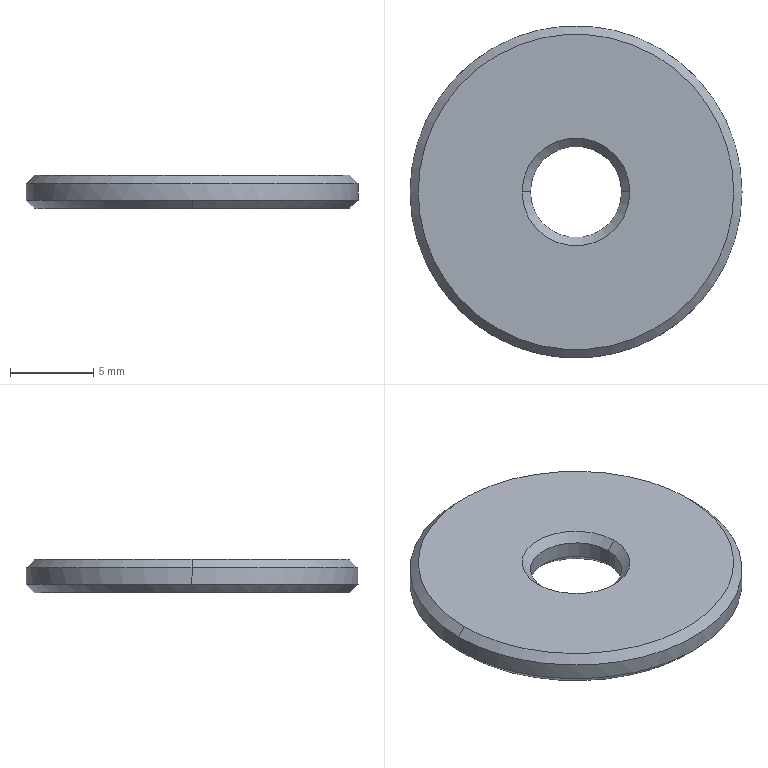Part | SolidWorks | features BaseBody 1 | 1 solid | 14 faces | box 20 x 20 x 2 mm | volume 560.774 mm3 | cone 8 | cylinder 4 | plane 2 | commonest cylinder face diameters 5.5 x2 20 x2
STEP:
#1=CARTESIAN_POINT('',(0.,9.5,-2.));
#2=VERTEX_POINT('',#1);
#3=CARTESIAN_POINT('',(0.,-9.5,-2.));
#4=VERTEX_POINT('',#3);
#5=CARTESIAN_POINT('',(0.,0.,-2.));
#6=DIRECTION('',(0.,0.,-1.));
#7=DIRECTION('',(0.,-1.,0.));
#8=AXIS2_PLACEMENT_3D('',#5,#6,#7);
#9=CIRCLE('',#8,9.5);
#10=EDGE_CURVE('',#2,#4,#9,.T.);
#11=ORIENTED_EDGE('',*,*,#10,.F.);
#12=CARTESIAN_POINT('',(0.,10.,-1.5));
#13=VERTEX_POINT('',#12);
#14=CARTESIAN_POINT('',(0.,10.,-1.5));
#15=DIRECTION('',(0.,0.7071,0.7071));
#16=VECTOR('',#15,1000.);
#17=LINE('',#14,#16);
#18=EDGE_CURVE('',#2,#13,#17,.T.);
#19=ORIENTED_EDGE('',*,*,#18,.T.);
#20=CARTESIAN_POINT('',(10.,0.,-1.5));
#21=VERTEX_POINT('',#20);
#22=CARTESIAN_POINT('',(0.,0.,-1.5));
#23=DIRECTION('',(0.,0.,-1.));
#24=DIRECTION('',(1.,0.,0.));
#25=AXIS2_PLACEMENT_3D('',#22,#23,#24);
#26=CIRCLE('',#25,10.);
#27=EDGE_CURVE('',#13,#21,#26,.T.);
#28=ORIENTED_EDGE('',*,*,#27,.T.);
#29=CARTESIAN_POINT('',(0.,-10.,-1.5));
#30=VERTEX_POINT('',#29);
#31=CARTESIAN_POINT('',(0.,0.,-1.5));
#32=DIRECTION('',(0.,0.,-1.));
#33=DIRECTION('',(1.,0.,0.));
#34=AXIS2_PLACEMENT_3D('',#31,#32,#33);
#35=CIRCLE('',#34,10.);
#36=EDGE_CURVE('',#21,#30,#35,.T.);
#37=ORIENTED_EDGE('',*,*,#36,.T.);
#38=CARTESIAN_POINT('',(0.,-10.,-1.5));
#39=DIRECTION('',(0.,-0.7071,0.7071));
#40=VECTOR('',#39,1000.);
#41=LINE('',#38,#40);
#42=EDGE_CURVE('',#4,#30,#41,.T.);
#43=ORIENTED_EDGE('',*,*,#42,.F.);
#44=EDGE_LOOP('',(#11,#19,#28,#37,#43));
#45=FACE_OUTER_BOUND('',#44,.T.);
#46=CARTESIAN_POINT('',(0.,0.,-1.5));
#47=DIRECTION('',(0.,0.,1.));
#48=DIRECTION('',(0.,-1.,0.));
#49=AXIS2_PLACEMENT_3D('',#46,#47,#48);
#50=CONICAL_SURFACE('',#49,10.,0.7854);
#51=ADVANCED_FACE('',(#45),#50,.T.);
#52=CARTESIAN_POINT('',(2.75,0.,-1.5));
#53=VERTEX_POINT('',#52);
#54=CARTESIAN_POINT('',(-2.75,0.,-1.5));
#55=VERTEX_POINT('',#54);
#56=CARTESIAN_POINT('',(0.,0.,-1.5));
#57=DIRECTION('',(0.,0.,-1.));
#58=DIRECTION('',(1.,0.,0.));
#59=AXIS2_PLACEMENT_3D('',#56,#57,#58);
#60=CIRCLE('',#59,2.75);
#61=EDGE_CURVE('',#53,#55,#60,.T.);
#62=ORIENTED_EDGE('',*,*,#61,.F.);
#63=CARTESIAN_POINT('',(3.25,0.,-2.));
#64=VERTEX_POINT('',#63);
#65=CARTESIAN_POINT('',(3.25,0.,-2.));
#66=DIRECTION('',(0.7071,0.,-0.7071));
#67=VECTOR('',#66,1000.);
#68=LINE('',#65,#67);
#69=EDGE_CURVE('',#53,#64,#68,.T.);
#70=ORIENTED_EDGE('',*,*,#69,.T.);
#71=CARTESIAN_POINT('',(-3.25,0.,-2.));
#72=VERTEX_POINT('',#71);
#73=CARTESIAN_POINT('',(0.,0.,-2.));
#74=DIRECTION('',(0.,0.,1.));
#75=DIRECTION('',(-1.,0.,0.));
#76=AXIS2_PLACEMENT_3D('',#73,#74,#75);
#77=CIRCLE('',#76,3.25);
#78=EDGE_CURVE('',#72,#64,#77,.T.);
#79=ORIENTED_EDGE('',*,*,#78,.F.);
#80=CARTESIAN_POINT('',(-3.25,0.,-2.));
#81=DIRECTION('',(-0.7071,0.,-0.7071));
#82=VECTOR('',#81,1000.);
#83=LINE('',#80,#82);
#84=EDGE_CURVE('',#55,#72,#83,.T.);
#85=ORIENTED_EDGE('',*,*,#84,.F.);
#86=EDGE_LOOP('',(#62,#70,#79,#85));
#87=FACE_OUTER_BOUND('',#86,.T.);
#88=CARTESIAN_POINT('',(0.,0.,-2.));
#89=DIRECTION('',(0.,0.,-1.));
#90=DIRECTION('',(-1.,0.,0.));
#91=AXIS2_PLACEMENT_3D('',#88,#89,#90);
#92=CONICAL_SURFACE('',#91,3.25,0.7854);
#93=ADVANCED_FACE('',(#87),#92,.F.);
#94=CARTESIAN_POINT('',(-10.,0.,-1.5));
#95=VERTEX_POINT('',#94);
#96=CARTESIAN_POINT('',(0.,0.,-1.5));
#97=DIRECTION('',(0.,0.,-1.));
#98=DIRECTION('',(1.,0.,0.));
#99=AXIS2_PLACEMENT_3D('',#96,#97,#98);
#100=CIRCLE('',#99,10.);
#101=EDGE_CURVE('',#95,#13,#100,.T.);
#102=ORIENTED_EDGE('',*,*,#101,.F.);
#103=CARTESIAN_POINT('',(-10.,0.,-0.5));
#104=VERTEX_POINT('',#103);
#105=CARTESIAN_POINT('',(-10.,0.,-1.));
#106=DIRECTION('',(0.,0.,1.));
#107=VECTOR('',#106,1000.);
#108=LINE('',#105,#107);
#109=EDGE_CURVE('',#95,#104,#108,.T.);
#110=ORIENTED_EDGE('',*,*,#109,.T.);
#111=CARTESIAN_POINT('',(10.,0.,-0.5));
#112=VERTEX_POINT('',#111);
#113=CARTESIAN_POINT('',(0.,0.,-0.5));
#114=DIRECTION('',(0.,0.,-1.));
#115=DIRECTION('',(1.,0.,0.));
#116=AXIS2_PLACEMENT_3D('',#113,#114,#115);
#117=CIRCLE('',#116,10.);
#118=EDGE_CURVE('',#104,#112,#117,.T.);
#119=ORIENTED_EDGE('',*,*,#118,.T.);
#120=CARTESIAN_POINT('',(10.,0.,-1.));
#121=DIRECTION('',(0.,0.,1.));
#122=VECTOR('',#121,1000.);
#123=LINE('',#120,#122);
#124=EDGE_CURVE('',#21,#112,#123,.T.);
#125=ORIENTED_EDGE('',*,*,#124,.F.);
#126=ORIENTED_EDGE('',*,*,#27,.F.);
#127=EDGE_LOOP('',(#102,#110,#119,#125,#126));
#128=FACE_OUTER_BOUND('',#127,.T.);
#129=CARTESIAN_POINT('',(0.,0.,-1.));
#130=DIRECTION('',(0.,0.,1.));
#131=DIRECTION('',(1.,0.,0.));
#132=AXIS2_PLACEMENT_3D('',#129,#130,#131);
#133=CYLINDRICAL_SURFACE('',#132,10.);
#134=ADVANCED_FACE('',(#128),#133,.T.);
#135=ORIENTED_EDGE('',*,*,#61,.T.);
#136=CARTESIAN_POINT('',(-2.75,0.,-0.5));
#137=VERTEX_POINT('',#136);
#138=CARTESIAN_POINT('',(-2.75,0.,-1.));
#139=DIRECTION('',(0.,0.,1.));
#140=VECTOR('',#139,1000.);
#141=LINE('',#138,#140);
#142=EDGE_CURVE('',#55,#137,#141,.T.);
#143=ORIENTED_EDGE('',*,*,#142,.T.);
#144=CARTESIAN_POINT('',(2.75,0.,-0.5));
#145=VERTEX_POINT('',#144);
#146=CARTESIAN_POINT('',(0.,0.,-0.5));
#147=DIRECTION('',(0.,0.,-1.));
#148=DIRECTION('',(1.,0.,0.));
#149=AXIS2_PLACEMENT_3D('',#146,#147,#148);
#150=CIRCLE('',#149,2.75);
#151=EDGE_CURVE('',#145,#137,#150,.T.);
#152=ORIENTED_EDGE('',*,*,#151,.F.);
#153=CARTESIAN_POINT('',(2.75,0.,-1.));
#154=DIRECTION('',(0.,0.,1.));
#155=VECTOR('',#154,1000.);
#156=LINE('',#153,#155);
#157=EDGE_CURVE('',#53,#145,#156,.T.);
#158=ORIENTED_EDGE('',*,*,#157,.F.);
#159=EDGE_LOOP('',(#135,#143,#152,#158));
#160=FACE_OUTER_BOUND('',#159,.T.);
#161=CARTESIAN_POINT('',(0.,0.,-1.));
#162=DIRECTION('',(0.,0.,1.));
#163=DIRECTION('',(1.,0.,0.));
#164=AXIS2_PLACEMENT_3D('',#161,#162,#163);
#165=CYLINDRICAL_SURFACE('',#164,2.75);
#166=ADVANCED_FACE('',(#160),#165,.F.);
#167=CARTESIAN_POINT('',(-9.5,0.,0.));
#168=VERTEX_POINT('',#167);
#169=CARTESIAN_POINT('',(9.5,0.,0.));
#170=VERTEX_POINT('',#169);
#171=CARTESIAN_POINT('',(0.,0.,0.));
#172=DIRECTION('',(0.,0.,-1.));
#173=DIRECTION('',(-1.,0.,0.));
#174=AXIS2_PLACEMENT_3D('',#171,#172,#173);
#175=CIRCLE('',#174,9.5);
#176=EDGE_CURVE('',#168,#170,#175,.T.);
#177=ORIENTED_EDGE('',*,*,#176,.T.);
#178=CARTESIAN_POINT('',(10.,0.,-0.5));
#179=DIRECTION('',(0.7071,0.,-0.7071));
#180=VECTOR('',#179,1000.);
#181=LINE('',#178,#180);
#182=EDGE_CURVE('',#170,#112,#181,.T.);
#183=ORIENTED_EDGE('',*,*,#182,.T.);
#184=ORIENTED_EDGE('',*,*,#118,.F.);
#185=CARTESIAN_POINT('',(-10.,0.,-0.5));
#186=DIRECTION('',(-0.7071,0.,-0.7071));
#187=VECTOR('',#186,1000.);
#188=LINE('',#185,#187);
#189=EDGE_CURVE('',#168,#104,#188,.T.);
#190=ORIENTED_EDGE('',*,*,#189,.F.);
#191=EDGE_LOOP('',(#177,#183,#184,#190));
#192=FACE_OUTER_BOUND('',#191,.T.);
#193=CARTESIAN_POINT('',(0.,0.,-0.5));
#194=DIRECTION('',(0.,0.,-1.));
#195=DIRECTION('',(-1.,0.,0.));
#196=AXIS2_PLACEMENT_3D('',#193,#194,#195);
#197=CONICAL_SURFACE('',#196,10.,0.7854);
#198=ADVANCED_FACE('',(#192),#197,.T.);
#199=ORIENTED_EDGE('',*,*,#151,.T.);
#200=CARTESIAN_POINT('',(-3.25,0.,0.));
#201=VERTEX_POINT('',#200);
#202=CARTESIAN_POINT('',(-3.25,0.,0.));
#203=DIRECTION('',(-0.7071,0.,0.7071));
#204=VECTOR('',#203,1000.);
#205=LINE('',#202,#204);
#206=EDGE_CURVE('',#137,#201,#205,.T.);
#207=ORIENTED_EDGE('',*,*,#206,.T.);
#208=CARTESIAN_POINT('',(3.25,0.,0.));
#209=VERTEX_POINT('',#208);
#210=CARTESIAN_POINT('',(0.,0.,0.));
#211=DIRECTION('',(0.,0.,-1.));
#212=DIRECTION('',(1.,0.,0.));
#213=AXIS2_PLACEMENT_3D('',#210,#211,#212);
#214=CIRCLE('',#213,3.25);
#215=EDGE_CURVE('',#209,#201,#214,.T.);
#216=ORIENTED_EDGE('',*,*,#215,.F.);
#217=CARTESIAN_POINT('',(3.25,0.,0.));
#218=DIRECTION('',(0.7071,0.,0.7071));
#219=VECTOR('',#218,1000.);
#220=LINE('',#217,#219);
#221=EDGE_CURVE('',#145,#209,#220,.T.);
#222=ORIENTED_EDGE('',*,*,#221,.F.);
#223=EDGE_LOOP('',(#199,#207,#216,#222));
#224=FACE_OUTER_BOUND('',#223,.T.);
#225=CARTESIAN_POINT('',(0.,0.,0.));
#226=DIRECTION('',(0.,0.,1.));
#227=DIRECTION('',(1.,0.,0.));
#228=AXIS2_PLACEMENT_3D('',#225,#226,#227);
#229=CONICAL_SURFACE('',#228,3.25,0.7854);
#230=ADVANCED_FACE('',(#224),#229,.F.);
#231=CARTESIAN_POINT('',(0.,0.,-2.));
#232=DIRECTION('',(0.,0.,-1.));
#233=DIRECTION('',(0.,-1.,0.));
#234=AXIS2_PLACEMENT_3D('',#231,#232,#233);
#235=CIRCLE('',#234,9.5);
#236=EDGE_CURVE('',#4,#2,#235,.T.);
#237=ORIENTED_EDGE('',*,*,#236,.T.);
#238=ORIENTED_EDGE('',*,*,#10,.T.);
#239=EDGE_LOOP('',(#237,#238));
#240=FACE_OUTER_BOUND('',#239,.T.);
#241=ORIENTED_EDGE('',*,*,#78,.T.);
#242=CARTESIAN_POINT('',(0.,0.,-2.));
#243=DIRECTION('',(0.,0.,1.));
#244=DIRECTION('',(-1.,0.,0.));
#245=AXIS2_PLACEMENT_3D('',#242,#243,#244);
#246=CIRCLE('',#245,3.25);
#247=EDGE_CURVE('',#64,#72,#246,.T.);
#248=ORIENTED_EDGE('',*,*,#247,.T.);
#249=EDGE_LOOP('',(#241,#248));
#250=FACE_BOUND('',#249,.T.);
#251=CARTESIAN_POINT('',(4.75,0.,-2.));
#252=DIRECTION('',(0.,0.,-1.));
#253=DIRECTION('',(-1.,0.,0.));
#254=AXIS2_PLACEMENT_3D('',#251,#252,#253);
#255=PLANE('',#254);
#256=ADVANCED_FACE('',(#240,#250),#255,.T.);
#257=ORIENTED_EDGE('',*,*,#18,.F.);
#258=ORIENTED_EDGE('',*,*,#236,.F.);
#259=ORIENTED_EDGE('',*,*,#42,.T.);
#260=CARTESIAN_POINT('',(0.,0.,-1.5));
#261=DIRECTION('',(0.,0.,-1.));
#262=DIRECTION('',(1.,0.,0.));
#263=AXIS2_PLACEMENT_3D('',#260,#261,#262);
#264=CIRCLE('',#263,10.);
#265=EDGE_CURVE('',#30,#95,#264,.T.);
#266=ORIENTED_EDGE('',*,*,#265,.T.);
#267=ORIENTED_EDGE('',*,*,#101,.T.);
#268=EDGE_LOOP('',(#257,#258,#259,#266,#267));
#269=FACE_OUTER_BOUND('',#268,.T.);
#270=CARTESIAN_POINT('',(0.,0.,-1.5));
#271=DIRECTION('',(0.,0.,1.));
#272=DIRECTION('',(0.,-1.,0.));
#273=AXIS2_PLACEMENT_3D('',#270,#271,#272);
#274=CONICAL_SURFACE('',#273,10.,0.7854);
#275=ADVANCED_FACE('',(#269),#274,.T.);
#276=ORIENTED_EDGE('',*,*,#69,.F.);
#277=CARTESIAN_POINT('',(0.,0.,-1.5));
#278=DIRECTION('',(0.,0.,-1.));
#279=DIRECTION('',(1.,0.,0.));
#280=AXIS2_PLACEMENT_3D('',#277,#278,#279);
#281=CIRCLE('',#280,2.75);
#282=EDGE_CURVE('',#55,#53,#281,.T.);
#283=ORIENTED_EDGE('',*,*,#282,.F.);
#284=ORIENTED_EDGE('',*,*,#84,.T.);
#285=ORIENTED_EDGE('',*,*,#247,.F.);
#286=EDGE_LOOP('',(#276,#283,#284,#285));
#287=FACE_OUTER_BOUND('',#286,.T.);
#288=CARTESIAN_POINT('',(0.,0.,-2.));
#289=DIRECTION('',(0.,0.,-1.));
#290=DIRECTION('',(-1.,0.,0.));
#291=AXIS2_PLACEMENT_3D('',#288,#289,#290);
#292=CONICAL_SURFACE('',#291,3.25,0.7854);
#293=ADVANCED_FACE('',(#287),#292,.F.);
#294=ORIENTED_EDGE('',*,*,#109,.F.);
#295=ORIENTED_EDGE('',*,*,#265,.F.);
#296=ORIENTED_EDGE('',*,*,#36,.F.);
#297=ORIENTED_EDGE('',*,*,#124,.T.);
#298=CARTESIAN_POINT('',(0.,0.,-0.5));
#299=DIRECTION('',(0.,0.,-1.));
#300=DIRECTION('',(1.,0.,0.));
#301=AXIS2_PLACEMENT_3D('',#298,#299,#300);
#302=CIRCLE('',#301,10.);
#303=EDGE_CURVE('',#112,#104,#302,.T.);
#304=ORIENTED_EDGE('',*,*,#303,.T.);
#305=EDGE_LOOP('',(#294,#295,#296,#297,#304));
#306=FACE_OUTER_BOUND('',#305,.T.);
#307=CARTESIAN_POINT('',(0.,0.,-1.));
#308=DIRECTION('',(0.,0.,1.));
#309=DIRECTION('',(1.,0.,0.));
#310=AXIS2_PLACEMENT_3D('',#307,#308,#309);
#311=CYLINDRICAL_SURFACE('',#310,10.);
#312=ADVANCED_FACE('',(#306),#311,.T.);
#313=ORIENTED_EDGE('',*,*,#142,.F.);
#314=ORIENTED_EDGE('',*,*,#282,.T.);
#315=ORIENTED_EDGE('',*,*,#157,.T.);
#316=CARTESIAN_POINT('',(0.,0.,-0.5));
#317=DIRECTION('',(0.,0.,-1.));
#318=DIRECTION('',(1.,0.,0.));
#319=AXIS2_PLACEMENT_3D('',#316,#317,#318);
#320=CIRCLE('',#319,2.75);
#321=EDGE_CURVE('',#137,#145,#320,.T.);
#322=ORIENTED_EDGE('',*,*,#321,.F.);
#323=EDGE_LOOP('',(#313,#314,#315,#322));
#324=FACE_OUTER_BOUND('',#323,.T.);
#325=CARTESIAN_POINT('',(0.,0.,-1.));
#326=DIRECTION('',(0.,0.,1.));
#327=DIRECTION('',(1.,0.,0.));
#328=AXIS2_PLACEMENT_3D('',#325,#326,#327);
#329=CYLINDRICAL_SURFACE('',#328,2.75);
#330=ADVANCED_FACE('',(#324),#329,.F.);
#331=ORIENTED_EDGE('',*,*,#182,.F.);
#332=CARTESIAN_POINT('',(0.,0.,0.));
#333=DIRECTION('',(0.,0.,-1.));
#334=DIRECTION('',(-1.,0.,0.));
#335=AXIS2_PLACEMENT_3D('',#332,#333,#334);
#336=CIRCLE('',#335,9.5);
#337=EDGE_CURVE('',#170,#168,#336,.T.);
#338=ORIENTED_EDGE('',*,*,#337,.T.);
#339=ORIENTED_EDGE('',*,*,#189,.T.);
#340=ORIENTED_EDGE('',*,*,#303,.F.);
#341=EDGE_LOOP('',(#331,#338,#339,#340));
#342=FACE_OUTER_BOUND('',#341,.T.);
#343=CARTESIAN_POINT('',(0.,0.,-0.5));
#344=DIRECTION('',(0.,0.,-1.));
#345=DIRECTION('',(-1.,0.,0.));
#346=AXIS2_PLACEMENT_3D('',#343,#344,#345);
#347=CONICAL_SURFACE('',#346,10.,0.7854);
#348=ADVANCED_FACE('',(#342),#347,.T.);
#349=ORIENTED_EDGE('',*,*,#206,.F.);
#350=ORIENTED_EDGE('',*,*,#321,.T.);
#351=ORIENTED_EDGE('',*,*,#221,.T.);
#352=CARTESIAN_POINT('',(0.,0.,0.));
#353=DIRECTION('',(0.,0.,-1.));
#354=DIRECTION('',(1.,0.,0.));
#355=AXIS2_PLACEMENT_3D('',#352,#353,#354);
#356=CIRCLE('',#355,3.25);
#357=EDGE_CURVE('',#201,#209,#356,.T.);
#358=ORIENTED_EDGE('',*,*,#357,.F.);
#359=EDGE_LOOP('',(#349,#350,#351,#358));
#360=FACE_OUTER_BOUND('',#359,.T.);
#361=CARTESIAN_POINT('',(0.,0.,0.));
#362=DIRECTION('',(0.,0.,1.));
#363=DIRECTION('',(1.,0.,0.));
#364=AXIS2_PLACEMENT_3D('',#361,#362,#363);
#365=CONICAL_SURFACE('',#364,3.25,0.7854);
#366=ADVANCED_FACE('',(#360),#365,.F.);
#367=ORIENTED_EDGE('',*,*,#176,.F.);
#368=ORIENTED_EDGE('',*,*,#337,.F.);
#369=EDGE_LOOP('',(#367,#368));
#370=FACE_OUTER_BOUND('',#369,.T.);
#371=ORIENTED_EDGE('',*,*,#215,.T.);
#372=ORIENTED_EDGE('',*,*,#357,.T.);
#373=EDGE_LOOP('',(#371,#372));
#374=FACE_BOUND('',#373,.T.);
#375=CARTESIAN_POINT('',(4.75,0.,0.));
#376=DIRECTION('',(0.,0.,1.));
#377=DIRECTION('',(1.,0.,0.));
#378=AXIS2_PLACEMENT_3D('',#375,#376,#377);
#379=PLANE('',#378);
#380=ADVANCED_FACE('',(#370,#374),#379,.T.);
#381=CLOSED_SHELL('',(#51,#93,#134,#166,#198,#230,#256,#275,#293,#312,#330,#348,#366,#380));
#382=MANIFOLD_SOLID_BREP('',#381);
#383=CARTESIAN_POINT('',(0.,0.,0.));
#384=DIRECTION('',(0.,0.,1.));
#385=DIRECTION('',(1.,0.,0.));
#386=AXIS2_PLACEMENT_3D('',#383,#384,#385);
#387=(LENGTH_UNIT()NAMED_UNIT(*)SI_UNIT(.MILLI.,.METRE.));
#388=UNCERTAINTY_MEASURE_WITH_UNIT(LENGTH_MEASURE(0.00001),#387,'','');
#389=(NAMED_UNIT(*)PLANE_ANGLE_UNIT()SI_UNIT($,.RADIAN.));
#390=(NAMED_UNIT(*)SI_UNIT($,.STERADIAN.)SOLID_ANGLE_UNIT());
#391=(GEOMETRIC_REPRESENTATION_CONTEXT(3)GLOBAL_UNCERTAINTY_ASSIGNED_CONTEXT((#388))GLOBAL_UNIT_ASSIGNED_CONTEXT((#387,#389,#390))REPRESENTATION_CONTEXT('',''));
#392=ADVANCED_BREP_SHAPE_REPRESENTATION('',(#382,#386),#391);